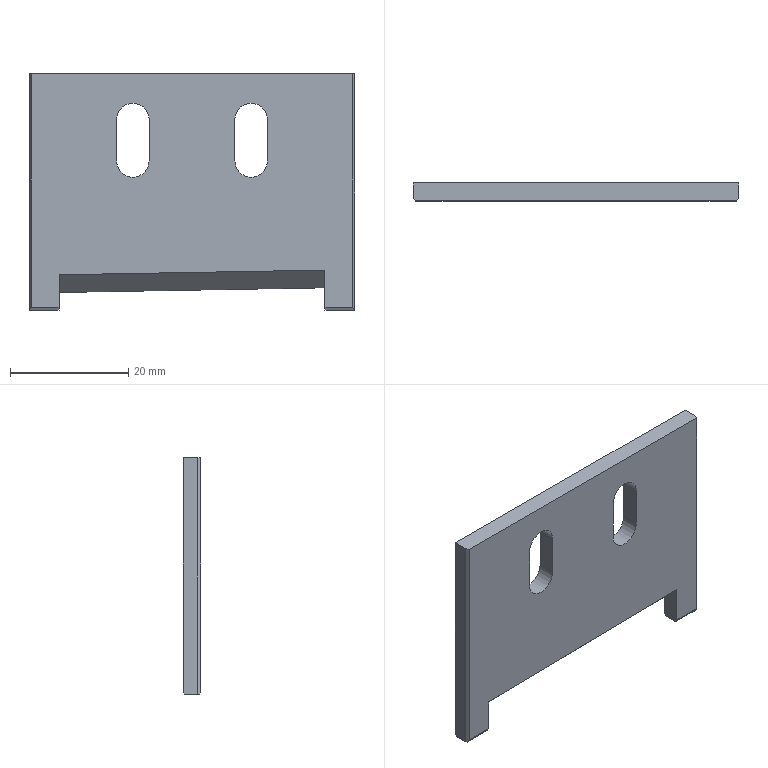Part | SolidWorks | features Chamfer 4, Draft 1, Extrusion 1, ICE 1 | 1 solid | 26 faces | box 55 x 3 x 40 mm | volume 5559 mm3 | plane 20 | cylinder 6 | commonest cylinder face diameters 5.5 x6
STEP:
#1=CARTESIAN_POINT('',(17.5,0.,-5.));
#2=VERTEX_POINT('',#1);
#3=CARTESIAN_POINT('',(20.25,0.,-7.75));
#4=VERTEX_POINT('',#3);
#5=CARTESIAN_POINT('',(17.5,0.,-7.75));
#6=DIRECTION('',(0.,1.,0.));
#7=DIRECTION('',(0.,0.,1.));
#8=AXIS2_PLACEMENT_3D('',#5,#6,#7);
#9=CIRCLE('',#8,2.75);
#10=EDGE_CURVE('',#2,#4,#9,.T.);
#11=ORIENTED_EDGE('',*,*,#10,.F.);
#12=CARTESIAN_POINT('',(17.5,3.,-5.));
#13=VERTEX_POINT('',#12);
#14=CARTESIAN_POINT('',(17.5,0.,-5.));
#15=DIRECTION('',(0.,1.,0.));
#16=VECTOR('',#15,1000.);
#17=LINE('',#14,#16);
#18=EDGE_CURVE('',#2,#13,#17,.T.);
#19=ORIENTED_EDGE('',*,*,#18,.T.);
#20=CARTESIAN_POINT('',(20.25,3.,-7.75));
#21=VERTEX_POINT('',#20);
#22=CARTESIAN_POINT('',(17.5,3.,-7.75));
#23=DIRECTION('',(0.,1.,0.));
#24=DIRECTION('',(0.,0.,1.));
#25=AXIS2_PLACEMENT_3D('',#22,#23,#24);
#26=CIRCLE('',#25,2.75);
#27=EDGE_CURVE('',#13,#21,#26,.T.);
#28=ORIENTED_EDGE('',*,*,#27,.T.);
#29=CARTESIAN_POINT('',(20.25,0.,-7.75));
#30=DIRECTION('',(0.,1.,0.));
#31=VECTOR('',#30,1000.);
#32=LINE('',#29,#31);
#33=EDGE_CURVE('',#4,#21,#32,.T.);
#34=ORIENTED_EDGE('',*,*,#33,.F.);
#35=EDGE_LOOP('',(#11,#19,#28,#34));
#36=FACE_OUTER_BOUND('',#35,.T.);
#37=CARTESIAN_POINT('',(17.5,0.,-7.75));
#38=DIRECTION('',(0.,1.,0.));
#39=DIRECTION('',(0.,0.,1.));
#40=AXIS2_PLACEMENT_3D('',#37,#38,#39);
#41=CYLINDRICAL_SURFACE('',#40,2.75);
#42=ADVANCED_FACE('',(#36),#41,.F.);
#43=CARTESIAN_POINT('',(37.5,0.,-5.));
#44=VERTEX_POINT('',#43);
#45=CARTESIAN_POINT('',(40.25,0.,-7.75));
#46=VERTEX_POINT('',#45);
#47=CARTESIAN_POINT('',(37.5,0.,-7.75));
#48=DIRECTION('',(0.,1.,0.));
#49=DIRECTION('',(0.,0.,1.));
#50=AXIS2_PLACEMENT_3D('',#47,#48,#49);
#51=CIRCLE('',#50,2.75);
#52=EDGE_CURVE('',#44,#46,#51,.T.);
#53=ORIENTED_EDGE('',*,*,#52,.F.);
#54=CARTESIAN_POINT('',(37.5,3.,-5.));
#55=VERTEX_POINT('',#54);
#56=CARTESIAN_POINT('',(37.5,0.,-5.));
#57=DIRECTION('',(0.,1.,0.));
#58=VECTOR('',#57,1000.);
#59=LINE('',#56,#58);
#60=EDGE_CURVE('',#44,#55,#59,.T.);
#61=ORIENTED_EDGE('',*,*,#60,.T.);
#62=CARTESIAN_POINT('',(40.25,3.,-7.75));
#63=VERTEX_POINT('',#62);
#64=CARTESIAN_POINT('',(37.5,3.,-7.75));
#65=DIRECTION('',(0.,1.,0.));
#66=DIRECTION('',(0.,0.,1.));
#67=AXIS2_PLACEMENT_3D('',#64,#65,#66);
#68=CIRCLE('',#67,2.75);
#69=EDGE_CURVE('',#55,#63,#68,.T.);
#70=ORIENTED_EDGE('',*,*,#69,.T.);
#71=CARTESIAN_POINT('',(40.25,0.,-7.75));
#72=DIRECTION('',(0.,1.,0.));
#73=VECTOR('',#72,1000.);
#74=LINE('',#71,#73);
#75=EDGE_CURVE('',#46,#63,#74,.T.);
#76=ORIENTED_EDGE('',*,*,#75,.F.);
#77=EDGE_LOOP('',(#53,#61,#70,#76));
#78=FACE_OUTER_BOUND('',#77,.T.);
#79=CARTESIAN_POINT('',(37.5,0.,-7.75));
#80=DIRECTION('',(0.,1.,0.));
#81=DIRECTION('',(0.,0.,1.));
#82=AXIS2_PLACEMENT_3D('',#79,#80,#81);
#83=CYLINDRICAL_SURFACE('',#82,2.75);
#84=ADVANCED_FACE('',(#78),#83,.F.);
#85=CARTESIAN_POINT('',(0.2887,0.,0.));
#86=VERTEX_POINT('',#85);
#87=CARTESIAN_POINT('',(54.711,0.,0.));
#88=VERTEX_POINT('',#87);
#89=CARTESIAN_POINT('',(0.,0.,0.));
#90=DIRECTION('',(1.,0.,0.));
#91=VECTOR('',#90,1000.);
#92=LINE('',#89,#91);
#93=EDGE_CURVE('',#86,#88,#92,.T.);
#94=ORIENTED_EDGE('',*,*,#93,.T.);
#95=CARTESIAN_POINT('',(55.,0.5,0.));
#96=VERTEX_POINT('',#95);
#97=CARTESIAN_POINT('',(55.,0.5,0.));
#98=DIRECTION('',(0.5,0.866,0.));
#99=VECTOR('',#98,1000.);
#100=LINE('',#97,#99);
#101=EDGE_CURVE('',#88,#96,#100,.T.);
#102=ORIENTED_EDGE('',*,*,#101,.T.);
#103=CARTESIAN_POINT('',(55.,3.,0.));
#104=VERTEX_POINT('',#103);
#105=CARTESIAN_POINT('',(55.,3.,0.));
#106=DIRECTION('',(0.,-1.,0.));
#107=VECTOR('',#106,1000.);
#108=LINE('',#105,#107);
#109=EDGE_CURVE('',#104,#96,#108,.T.);
#110=ORIENTED_EDGE('',*,*,#109,.F.);
#111=CARTESIAN_POINT('',(0.,3.,0.));
#112=VERTEX_POINT('',#111);
#113=CARTESIAN_POINT('',(0.,3.,0.));
#114=DIRECTION('',(1.,0.,0.));
#115=VECTOR('',#114,1000.);
#116=LINE('',#113,#115);
#117=EDGE_CURVE('',#112,#104,#116,.T.);
#118=ORIENTED_EDGE('',*,*,#117,.F.);
#119=CARTESIAN_POINT('',(0.,0.5,0.));
#120=VERTEX_POINT('',#119);
#121=CARTESIAN_POINT('',(0.,3.,0.));
#122=DIRECTION('',(0.,-1.,0.));
#123=VECTOR('',#122,1000.);
#124=LINE('',#121,#123);
#125=EDGE_CURVE('',#112,#120,#124,.T.);
#126=ORIENTED_EDGE('',*,*,#125,.T.);
#127=CARTESIAN_POINT('',(0.,0.5,0.));
#128=DIRECTION('',(0.5,-0.866,0.));
#129=VECTOR('',#128,1000.);
#130=LINE('',#127,#129);
#131=EDGE_CURVE('',#120,#86,#130,.T.);
#132=ORIENTED_EDGE('',*,*,#131,.T.);
#133=EDGE_LOOP('',(#94,#102,#110,#118,#126,#132));
#134=FACE_OUTER_BOUND('',#133,.T.);
#135=CARTESIAN_POINT('',(0.,3.,0.));
#136=DIRECTION('',(0.,0.,-1.));
#137=DIRECTION('',(-1.,0.,0.));
#138=AXIS2_PLACEMENT_3D('',#135,#136,#137);
#139=PLANE('',#138);
#140=ADVANCED_FACE('',(#134),#139,.F.);
#141=ORIENTED_EDGE('',*,*,#109,.T.);
#142=CARTESIAN_POINT('',(55.,0.5,-40.));
#143=VERTEX_POINT('',#142);
#144=CARTESIAN_POINT('',(55.,0.5,-39.5));
#145=DIRECTION('',(0.,0.,-1.));
#146=VECTOR('',#145,1000.);
#147=LINE('',#144,#146);
#148=EDGE_CURVE('',#96,#143,#147,.T.);
#149=ORIENTED_EDGE('',*,*,#148,.T.);
#150=CARTESIAN_POINT('',(55.,2.711,-40.));
#151=VERTEX_POINT('',#150);
#152=CARTESIAN_POINT('',(55.,3.,-40.));
#153=DIRECTION('',(0.,-1.,0.));
#154=VECTOR('',#153,1000.);
#155=LINE('',#152,#154);
#156=EDGE_CURVE('',#151,#143,#155,.T.);
#157=ORIENTED_EDGE('',*,*,#156,.F.);
#158=CARTESIAN_POINT('',(55.,3.,-39.5));
#159=VERTEX_POINT('',#158);
#160=CARTESIAN_POINT('',(55.,3.,-39.5));
#161=DIRECTION('',(0.,0.5,0.866));
#162=VECTOR('',#161,1000.);
#163=LINE('',#160,#162);
#164=EDGE_CURVE('',#151,#159,#163,.T.);
#165=ORIENTED_EDGE('',*,*,#164,.T.);
#166=CARTESIAN_POINT('',(55.,3.,0.));
#167=DIRECTION('',(0.,0.,-1.));
#168=VECTOR('',#167,1000.);
#169=LINE('',#166,#168);
#170=EDGE_CURVE('',#104,#159,#169,.T.);
#171=ORIENTED_EDGE('',*,*,#170,.F.);
#172=EDGE_LOOP('',(#141,#149,#157,#165,#171));
#173=FACE_OUTER_BOUND('',#172,.T.);
#174=CARTESIAN_POINT('',(55.,3.,-37.));
#175=DIRECTION('',(-1.,0.,0.));
#176=DIRECTION('',(0.,0.,1.));
#177=AXIS2_PLACEMENT_3D('',#174,#175,#176);
#178=PLANE('',#177);
#179=ADVANCED_FACE('',(#173),#178,.F.);
#180=ORIENTED_EDGE('',*,*,#156,.T.);
#181=CARTESIAN_POINT('',(54.878,0.2887,-40.));
#182=VERTEX_POINT('',#181);
#183=CARTESIAN_POINT('',(55.,0.5,-40.));
#184=DIRECTION('',(-0.5,-0.866,0.));
#185=VECTOR('',#184,1000.);
#186=LINE('',#183,#185);
#187=EDGE_CURVE('',#143,#182,#186,.T.);
#188=ORIENTED_EDGE('',*,*,#187,.T.);
#189=CARTESIAN_POINT('',(50.,0.2887,-40.));
#190=VERTEX_POINT('',#189);
#191=CARTESIAN_POINT('',(50.,0.2887,-40.));
#192=DIRECTION('',(-1.,0.,0.));
#193=VECTOR('',#192,1000.);
#194=LINE('',#191,#193);
#195=EDGE_CURVE('',#182,#190,#194,.T.);
#196=ORIENTED_EDGE('',*,*,#195,.T.);
#197=CARTESIAN_POINT('',(50.,2.711,-40.));
#198=VERTEX_POINT('',#197);
#199=CARTESIAN_POINT('',(50.,3.,-40.));
#200=DIRECTION('',(0.,-1.,0.));
#201=VECTOR('',#200,1000.);
#202=LINE('',#199,#201);
#203=EDGE_CURVE('',#198,#190,#202,.T.);
#204=ORIENTED_EDGE('',*,*,#203,.F.);
#205=CARTESIAN_POINT('',(55.,2.711,-40.));
#206=DIRECTION('',(1.,0.,0.));
#207=VECTOR('',#206,1000.);
#208=LINE('',#205,#207);
#209=EDGE_CURVE('',#198,#151,#208,.T.);
#210=ORIENTED_EDGE('',*,*,#209,.T.);
#211=EDGE_LOOP('',(#180,#188,#196,#204,#210));
#212=FACE_OUTER_BOUND('',#211,.T.);
#213=CARTESIAN_POINT('',(55.,3.,-40.));
#214=DIRECTION('',(0.,0.,1.));
#215=DIRECTION('',(1.,0.,0.));
#216=AXIS2_PLACEMENT_3D('',#213,#214,#215);
#217=PLANE('',#216);
#218=ADVANCED_FACE('',(#212),#217,.F.);
#219=CARTESIAN_POINT('',(50.,3.,-39.5));
#220=VERTEX_POINT('',#219);
#221=CARTESIAN_POINT('',(50.,3.,-36.215));
#222=VERTEX_POINT('',#221);
#223=CARTESIAN_POINT('',(50.,3.,-37.));
#224=DIRECTION('',(0.,0.,1.));
#225=VECTOR('',#224,1000.);
#226=LINE('',#223,#225);
#227=EDGE_CURVE('',#220,#222,#226,.T.);
#228=ORIENTED_EDGE('',*,*,#227,.F.);
#229=CARTESIAN_POINT('',(50.,3.,-39.5));
#230=DIRECTION('',(0.,-0.5,-0.866));
#231=VECTOR('',#230,1000.);
#232=LINE('',#229,#231);
#233=EDGE_CURVE('',#220,#198,#232,.T.);
#234=ORIENTED_EDGE('',*,*,#233,.T.);
#235=ORIENTED_EDGE('',*,*,#203,.T.);
#236=CARTESIAN_POINT('',(50.,0.,-39.5));
#237=VERTEX_POINT('',#236);
#238=CARTESIAN_POINT('',(50.,0.2887,-40.));
#239=DIRECTION('',(0.,-0.5,0.866));
#240=VECTOR('',#239,1000.);
#241=LINE('',#238,#240);
#242=EDGE_CURVE('',#190,#237,#241,.T.);
#243=ORIENTED_EDGE('',*,*,#242,.T.);
#244=CARTESIAN_POINT('',(50.,0.,-33.214));
#245=VERTEX_POINT('',#244);
#246=CARTESIAN_POINT('',(50.,0.,-37.));
#247=DIRECTION('',(0.,0.,1.));
#248=VECTOR('',#247,1000.);
#249=LINE('',#246,#248);
#250=EDGE_CURVE('',#237,#245,#249,.T.);
#251=ORIENTED_EDGE('',*,*,#250,.T.);
#252=CARTESIAN_POINT('',(50.,3.393,-36.607));
#253=DIRECTION('',(0.,0.7071,-0.7072));
#254=VECTOR('',#253,1000.);
#255=LINE('',#252,#254);
#256=EDGE_CURVE('',#245,#222,#255,.T.);
#257=ORIENTED_EDGE('',*,*,#256,.T.);
#258=EDGE_LOOP('',(#228,#234,#235,#243,#251,#257));
#259=FACE_OUTER_BOUND('',#258,.T.);
#260=CARTESIAN_POINT('',(50.,3.,-37.));
#261=DIRECTION('',(1.,0.,0.));
#262=DIRECTION('',(0.,0.,-1.));
#263=AXIS2_PLACEMENT_3D('',#260,#261,#262);
#264=PLANE('',#263);
#265=ADVANCED_FACE('',(#259),#264,.F.);
#266=CARTESIAN_POINT('',(5.,2.711,-40.));
#267=VERTEX_POINT('',#266);
#268=CARTESIAN_POINT('',(5.,0.2887,-40.));
#269=VERTEX_POINT('',#268);
#270=CARTESIAN_POINT('',(5.,3.,-40.));
#271=DIRECTION('',(0.,-1.,0.));
#272=VECTOR('',#271,1000.);
#273=LINE('',#270,#272);
#274=EDGE_CURVE('',#267,#269,#273,.T.);
#275=ORIENTED_EDGE('',*,*,#274,.F.);
#276=CARTESIAN_POINT('',(5.,3.,-39.5));
#277=VERTEX_POINT('',#276);
#278=CARTESIAN_POINT('',(5.,3.,-39.5));
#279=DIRECTION('',(0.,0.5,0.866));
#280=VECTOR('',#279,1000.);
#281=LINE('',#278,#280);
#282=EDGE_CURVE('',#267,#277,#281,.T.);
#283=ORIENTED_EDGE('',*,*,#282,.T.);
#284=CARTESIAN_POINT('',(5.,3.,-37.));
#285=VERTEX_POINT('',#284);
#286=CARTESIAN_POINT('',(5.,3.,-37.));
#287=DIRECTION('',(0.,0.,-1.));
#288=VECTOR('',#287,1000.);
#289=LINE('',#286,#288);
#290=EDGE_CURVE('',#285,#277,#289,.T.);
#291=ORIENTED_EDGE('',*,*,#290,.F.);
#292=CARTESIAN_POINT('',(5.,0.,-34.));
#293=VERTEX_POINT('',#292);
#294=CARTESIAN_POINT('',(5.,3.,-37.));
#295=DIRECTION('',(0.,-0.7071,0.7072));
#296=VECTOR('',#295,1000.);
#297=LINE('',#294,#296);
#298=EDGE_CURVE('',#285,#293,#297,.T.);
#299=ORIENTED_EDGE('',*,*,#298,.T.);
#300=CARTESIAN_POINT('',(5.,0.,-39.5));
#301=VERTEX_POINT('',#300);
#302=CARTESIAN_POINT('',(5.,0.,-37.));
#303=DIRECTION('',(0.,0.,-1.));
#304=VECTOR('',#303,1000.);
#305=LINE('',#302,#304);
#306=EDGE_CURVE('',#293,#301,#305,.T.);
#307=ORIENTED_EDGE('',*,*,#306,.T.);
#308=CARTESIAN_POINT('',(5.,0.2887,-40.));
#309=DIRECTION('',(0.,0.5,-0.866));
#310=VECTOR('',#309,1000.);
#311=LINE('',#308,#310);
#312=EDGE_CURVE('',#301,#269,#311,.T.);
#313=ORIENTED_EDGE('',*,*,#312,.T.);
#314=EDGE_LOOP('',(#275,#283,#291,#299,#307,#313));
#315=FACE_OUTER_BOUND('',#314,.T.);
#316=CARTESIAN_POINT('',(5.,3.,-37.));
#317=DIRECTION('',(-1.,0.,0.));
#318=DIRECTION('',(0.,0.,1.));
#319=AXIS2_PLACEMENT_3D('',#316,#317,#318);
#320=PLANE('',#319);
#321=ADVANCED_FACE('',(#315),#320,.F.);
#322=CARTESIAN_POINT('',(0.122,0.2887,-40.));
#323=VERTEX_POINT('',#322);
#324=CARTESIAN_POINT('',(0.,0.2887,-40.));
#325=DIRECTION('',(-1.,0.,0.));
#326=VECTOR('',#325,1000.);
#327=LINE('',#324,#326);
#328=EDGE_CURVE('',#269,#323,#327,.T.);
#329=ORIENTED_EDGE('',*,*,#328,.T.);
#330=CARTESIAN_POINT('',(0.,0.5,-40.));
#331=VERTEX_POINT('',#330);
#332=CARTESIAN_POINT('',(0.,0.5,-40.));
#333=DIRECTION('',(-0.5,0.866,0.));
#334=VECTOR('',#333,1000.);
#335=LINE('',#332,#334);
#336=EDGE_CURVE('',#323,#331,#335,.T.);
#337=ORIENTED_EDGE('',*,*,#336,.T.);
#338=CARTESIAN_POINT('',(0.,2.711,-40.));
#339=VERTEX_POINT('',#338);
#340=CARTESIAN_POINT('',(0.,3.,-40.));
#341=DIRECTION('',(0.,-1.,0.));
#342=VECTOR('',#341,1000.);
#343=LINE('',#340,#342);
#344=EDGE_CURVE('',#339,#331,#343,.T.);
#345=ORIENTED_EDGE('',*,*,#344,.F.);
#346=CARTESIAN_POINT('',(0.,2.711,-40.));
#347=DIRECTION('',(1.,0.,0.));
#348=VECTOR('',#347,1000.);
#349=LINE('',#346,#348);
#350=EDGE_CURVE('',#339,#267,#349,.T.);
#351=ORIENTED_EDGE('',*,*,#350,.T.);
#352=ORIENTED_EDGE('',*,*,#274,.T.);
#353=EDGE_LOOP('',(#329,#337,#345,#351,#352));
#354=FACE_OUTER_BOUND('',#353,.T.);
#355=CARTESIAN_POINT('',(0.,3.,-40.));
#356=DIRECTION('',(0.,0.,1.));
#357=DIRECTION('',(1.,0.,0.));
#358=AXIS2_PLACEMENT_3D('',#355,#356,#357);
#359=PLANE('',#358);
#360=ADVANCED_FACE('',(#354),#359,.F.);
#361=ORIENTED_EDGE('',*,*,#344,.T.);
#362=CARTESIAN_POINT('',(0.,0.5,0.));
#363=DIRECTION('',(0.,0.,1.));
#364=VECTOR('',#363,1000.);
#365=LINE('',#362,#364);
#366=EDGE_CURVE('',#331,#120,#365,.T.);
#367=ORIENTED_EDGE('',*,*,#366,.T.);
#368=ORIENTED_EDGE('',*,*,#125,.F.);
#369=CARTESIAN_POINT('',(0.,3.,-39.5));
#370=VERTEX_POINT('',#369);
#371=CARTESIAN_POINT('',(0.,3.,0.));
#372=DIRECTION('',(0.,0.,1.));
#373=VECTOR('',#372,1000.);
#374=LINE('',#371,#373);
#375=EDGE_CURVE('',#370,#112,#374,.T.);
#376=ORIENTED_EDGE('',*,*,#375,.F.);
#377=CARTESIAN_POINT('',(0.,3.,-39.5));
#378=DIRECTION('',(0.,-0.5,-0.866));
#379=VECTOR('',#378,1000.);
#380=LINE('',#377,#379);
#381=EDGE_CURVE('',#370,#339,#380,.T.);
#382=ORIENTED_EDGE('',*,*,#381,.T.);
#383=EDGE_LOOP('',(#361,#367,#368,#376,#382));
#384=FACE_OUTER_BOUND('',#383,.T.);
#385=CARTESIAN_POINT('',(0.,3.,-37.));
#386=DIRECTION('',(1.,0.,0.));
#387=DIRECTION('',(0.,0.,-1.));
#388=AXIS2_PLACEMENT_3D('',#385,#386,#387);
#389=PLANE('',#388);
#390=ADVANCED_FACE('',(#384),#389,.F.);
#391=CARTESIAN_POINT('',(14.75,3.,-14.75));
#392=VERTEX_POINT('',#391);
#393=CARTESIAN_POINT('',(14.75,3.,-7.75));
#394=VERTEX_POINT('',#393);
#395=CARTESIAN_POINT('',(14.75,3.,-14.75));
#396=DIRECTION('',(0.,0.,1.));
#397=VECTOR('',#396,1000.);
#398=LINE('',#395,#397);
#399=EDGE_CURVE('',#392,#394,#398,.T.);
#400=ORIENTED_EDGE('',*,*,#399,.F.);
#401=CARTESIAN_POINT('',(20.25,3.,-14.75));
#402=VERTEX_POINT('',#401);
#403=CARTESIAN_POINT('',(17.5,3.,-14.75));
#404=DIRECTION('',(0.,1.,0.));
#405=DIRECTION('',(0.,0.,1.));
#406=AXIS2_PLACEMENT_3D('',#403,#404,#405);
#407=CIRCLE('',#406,2.75);
#408=EDGE_CURVE('',#402,#392,#407,.T.);
#409=ORIENTED_EDGE('',*,*,#408,.F.);
#410=CARTESIAN_POINT('',(20.25,3.,-14.75));
#411=DIRECTION('',(0.,0.,-1.));
#412=VECTOR('',#411,1000.);
#413=LINE('',#410,#412);
#414=EDGE_CURVE('',#21,#402,#413,.T.);
#415=ORIENTED_EDGE('',*,*,#414,.F.);
#416=ORIENTED_EDGE('',*,*,#27,.F.);
#417=CARTESIAN_POINT('',(17.5,3.,-7.75));
#418=DIRECTION('',(0.,1.,0.));
#419=DIRECTION('',(0.,0.,1.));
#420=AXIS2_PLACEMENT_3D('',#417,#418,#419);
#421=CIRCLE('',#420,2.75);
#422=EDGE_CURVE('',#394,#13,#421,.T.);
#423=ORIENTED_EDGE('',*,*,#422,.F.);
#424=EDGE_LOOP('',(#400,#409,#415,#416,#423));
#425=FACE_BOUND('',#424,.T.);
#426=CARTESIAN_POINT('',(34.75,3.,-14.75));
#427=VERTEX_POINT('',#426);
#428=CARTESIAN_POINT('',(34.75,3.,-7.75));
#429=VERTEX_POINT('',#428);
#430=CARTESIAN_POINT('',(34.75,3.,-14.75));
#431=DIRECTION('',(0.,0.,1.));
#432=VECTOR('',#431,1000.);
#433=LINE('',#430,#432);
#434=EDGE_CURVE('',#427,#429,#433,.T.);
#435=ORIENTED_EDGE('',*,*,#434,.F.);
#436=CARTESIAN_POINT('',(40.25,3.,-14.75));
#437=VERTEX_POINT('',#436);
#438=CARTESIAN_POINT('',(37.5,3.,-14.75));
#439=DIRECTION('',(0.,1.,0.));
#440=DIRECTION('',(0.,0.,1.));
#441=AXIS2_PLACEMENT_3D('',#438,#439,#440);
#442=CIRCLE('',#441,2.75);
#443=EDGE_CURVE('',#437,#427,#442,.T.);
#444=ORIENTED_EDGE('',*,*,#443,.F.);
#445=CARTESIAN_POINT('',(40.25,3.,-14.75));
#446=DIRECTION('',(0.,0.,-1.));
#447=VECTOR('',#446,1000.);
#448=LINE('',#445,#447);
#449=EDGE_CURVE('',#63,#437,#448,.T.);
#450=ORIENTED_EDGE('',*,*,#449,.F.);
#451=ORIENTED_EDGE('',*,*,#69,.F.);
#452=CARTESIAN_POINT('',(37.5,3.,-7.75));
#453=DIRECTION('',(0.,1.,0.));
#454=DIRECTION('',(0.,0.,1.));
#455=AXIS2_PLACEMENT_3D('',#452,#453,#454);
#456=CIRCLE('',#455,2.75);
#457=EDGE_CURVE('',#429,#55,#456,.T.);
#458=ORIENTED_EDGE('',*,*,#457,.F.);
#459=EDGE_LOOP('',(#435,#444,#450,#451,#458));
#460=FACE_BOUND('',#459,.T.);
#461=ORIENTED_EDGE('',*,*,#290,.T.);
#462=CARTESIAN_POINT('',(0.,3.,-39.5));
#463=DIRECTION('',(-1.,0.,0.));
#464=VECTOR('',#463,1000.);
#465=LINE('',#462,#464);
#466=EDGE_CURVE('',#277,#370,#465,.T.);
#467=ORIENTED_EDGE('',*,*,#466,.T.);
#468=ORIENTED_EDGE('',*,*,#375,.T.);
#469=ORIENTED_EDGE('',*,*,#117,.T.);
#470=ORIENTED_EDGE('',*,*,#170,.T.);
#471=CARTESIAN_POINT('',(0.,3.,-39.5));
#472=DIRECTION('',(-1.,0.,0.));
#473=VECTOR('',#472,1000.);
#474=LINE('',#471,#473);
#475=EDGE_CURVE('',#159,#220,#474,.T.);
#476=ORIENTED_EDGE('',*,*,#475,.T.);
#477=ORIENTED_EDGE('',*,*,#227,.T.);
#478=CARTESIAN_POINT('',(0.6472,3.,-37.076));
#479=DIRECTION('',(-0.9998,0.,-0.01745));
#480=VECTOR('',#479,1000.);
#481=LINE('',#478,#480);
#482=EDGE_CURVE('',#222,#285,#481,.T.);
#483=ORIENTED_EDGE('',*,*,#482,.T.);
#484=EDGE_LOOP('',(#461,#467,#468,#469,#470,#476,#477,#483));
#485=FACE_OUTER_BOUND('',#484,.T.);
#486=CARTESIAN_POINT('',(0.,3.,0.));
#487=DIRECTION('',(0.,-1.,0.));
#488=DIRECTION('',(0.,0.,-1.));
#489=AXIS2_PLACEMENT_3D('',#486,#487,#488);
#490=PLANE('',#489);
#491=ADVANCED_FACE('',(#425,#460,#485),#490,.F.);
#492=CARTESIAN_POINT('',(20.25,0.,-14.75));
#493=VERTEX_POINT('',#492);
#494=CARTESIAN_POINT('',(14.75,0.,-14.75));
#495=VERTEX_POINT('',#494);
#496=CARTESIAN_POINT('',(17.5,0.,-14.75));
#497=DIRECTION('',(0.,1.,0.));
#498=DIRECTION('',(0.,0.,1.));
#499=AXIS2_PLACEMENT_3D('',#496,#497,#498);
#500=CIRCLE('',#499,2.75);
#501=EDGE_CURVE('',#493,#495,#500,.T.);
#502=ORIENTED_EDGE('',*,*,#501,.T.);
#503=CARTESIAN_POINT('',(14.75,0.,-7.75));
#504=VERTEX_POINT('',#503);
#505=CARTESIAN_POINT('',(14.75,0.,-14.75));
#506=DIRECTION('',(0.,0.,1.));
#507=VECTOR('',#506,1000.);
#508=LINE('',#505,#507);
#509=EDGE_CURVE('',#495,#504,#508,.T.);
#510=ORIENTED_EDGE('',*,*,#509,.T.);
#511=CARTESIAN_POINT('',(17.5,0.,-7.75));
#512=DIRECTION('',(0.,1.,0.));
#513=DIRECTION('',(0.,0.,1.));
#514=AXIS2_PLACEMENT_3D('',#511,#512,#513);
#515=CIRCLE('',#514,2.75);
#516=EDGE_CURVE('',#504,#2,#515,.T.);
#517=ORIENTED_EDGE('',*,*,#516,.T.);
#518=ORIENTED_EDGE('',*,*,#10,.T.);
#519=CARTESIAN_POINT('',(20.25,0.,-14.75));
#520=DIRECTION('',(0.,0.,-1.));
#521=VECTOR('',#520,1000.);
#522=LINE('',#519,#521);
#523=EDGE_CURVE('',#4,#493,#522,.T.);
#524=ORIENTED_EDGE('',*,*,#523,.T.);
#525=EDGE_LOOP('',(#502,#510,#517,#518,#524));
#526=FACE_BOUND('',#525,.T.);
#527=CARTESIAN_POINT('',(40.25,0.,-14.75));
#528=VERTEX_POINT('',#527);
#529=CARTESIAN_POINT('',(34.75,0.,-14.75));
#530=VERTEX_POINT('',#529);
#531=CARTESIAN_POINT('',(37.5,0.,-14.75));
#532=DIRECTION('',(0.,1.,0.));
#533=DIRECTION('',(0.,0.,1.));
#534=AXIS2_PLACEMENT_3D('',#531,#532,#533);
#535=CIRCLE('',#534,2.75);
#536=EDGE_CURVE('',#528,#530,#535,.T.);
#537=ORIENTED_EDGE('',*,*,#536,.T.);
#538=CARTESIAN_POINT('',(34.75,0.,-7.75));
#539=VERTEX_POINT('',#538);
#540=CARTESIAN_POINT('',(34.75,0.,-14.75));
#541=DIRECTION('',(0.,0.,1.));
#542=VECTOR('',#541,1000.);
#543=LINE('',#540,#542);
#544=EDGE_CURVE('',#530,#539,#543,.T.);
#545=ORIENTED_EDGE('',*,*,#544,.T.);
#546=CARTESIAN_POINT('',(37.5,0.,-7.75));
#547=DIRECTION('',(0.,1.,0.));
#548=DIRECTION('',(0.,0.,1.));
#549=AXIS2_PLACEMENT_3D('',#546,#547,#548);
#550=CIRCLE('',#549,2.75);
#551=EDGE_CURVE('',#539,#44,#550,.T.);
#552=ORIENTED_EDGE('',*,*,#551,.T.);
#553=ORIENTED_EDGE('',*,*,#52,.T.);
#554=CARTESIAN_POINT('',(40.25,0.,-14.75));
#555=DIRECTION('',(0.,0.,-1.));
#556=VECTOR('',#555,1000.);
#557=LINE('',#554,#556);
#558=EDGE_CURVE('',#46,#528,#557,.T.);
#559=ORIENTED_EDGE('',*,*,#558,.T.);
#560=EDGE_LOOP('',(#537,#545,#552,#553,#559));
#561=FACE_BOUND('',#560,.T.);
#562=CARTESIAN_POINT('',(54.711,0.,-39.5));
#563=VERTEX_POINT('',#562);
#564=CARTESIAN_POINT('',(55.,0.,-39.5));
#565=DIRECTION('',(1.,0.,0.));
#566=VECTOR('',#565,1000.);
#567=LINE('',#564,#566);
#568=EDGE_CURVE('',#237,#563,#567,.T.);
#569=ORIENTED_EDGE('',*,*,#568,.T.);
#570=CARTESIAN_POINT('',(54.711,0.,0.));
#571=DIRECTION('',(0.,0.,1.));
#572=VECTOR('',#571,1000.);
#573=LINE('',#570,#572);
#574=EDGE_CURVE('',#563,#88,#573,.T.);
#575=ORIENTED_EDGE('',*,*,#574,.T.);
#576=ORIENTED_EDGE('',*,*,#93,.F.);
#577=CARTESIAN_POINT('',(0.2887,0.,-39.5));
#578=VERTEX_POINT('',#577);
#579=CARTESIAN_POINT('',(0.2887,0.,-39.5));
#580=DIRECTION('',(0.,0.,-1.));
#581=VECTOR('',#580,1000.);
#582=LINE('',#579,#581);
#583=EDGE_CURVE('',#86,#578,#582,.T.);
#584=ORIENTED_EDGE('',*,*,#583,.T.);
#585=CARTESIAN_POINT('',(5.,0.,-39.5));
#586=DIRECTION('',(1.,0.,0.));
#587=VECTOR('',#586,1000.);
#588=LINE('',#585,#587);
#589=EDGE_CURVE('',#578,#301,#588,.T.);
#590=ORIENTED_EDGE('',*,*,#589,.T.);
#591=ORIENTED_EDGE('',*,*,#306,.F.);
#592=CARTESIAN_POINT('',(49.948,0.,-33.215));
#593=DIRECTION('',(0.9998,0.,0.01745));
#594=VECTOR('',#593,1000.);
#595=LINE('',#592,#594);
#596=EDGE_CURVE('',#293,#245,#595,.T.);
#597=ORIENTED_EDGE('',*,*,#596,.T.);
#598=ORIENTED_EDGE('',*,*,#250,.F.);
#599=EDGE_LOOP('',(#569,#575,#576,#584,#590,#591,#597,#598));
#600=FACE_OUTER_BOUND('',#599,.T.);
#601=CARTESIAN_POINT('',(0.,0.,0.));
#602=DIRECTION('',(0.,-1.,0.));
#603=DIRECTION('',(0.,0.,-1.));
#604=AXIS2_PLACEMENT_3D('',#601,#602,#603);
#605=PLANE('',#604);
#606=ADVANCED_FACE('',(#526,#561,#600),#605,.T.);
#607=ORIENTED_EDGE('',*,*,#443,.T.);
#608=CARTESIAN_POINT('',(34.75,0.,-14.75));
#609=DIRECTION('',(0.,1.,0.));
#610=VECTOR('',#609,1000.);
#611=LINE('',#608,#610);
#612=EDGE_CURVE('',#530,#427,#611,.T.);
#613=ORIENTED_EDGE('',*,*,#612,.F.);
#614=ORIENTED_EDGE('',*,*,#536,.F.);
#615=CARTESIAN_POINT('',(40.25,0.,-14.75));
#616=DIRECTION('',(0.,1.,0.));
#617=VECTOR('',#616,1000.);
#618=LINE('',#615,#617);
#619=EDGE_CURVE('',#528,#437,#618,.T.);
#620=ORIENTED_EDGE('',*,*,#619,.T.);
#621=EDGE_LOOP('',(#607,#613,#614,#620));
#622=FACE_OUTER_BOUND('',#621,.T.);
#623=CARTESIAN_POINT('',(37.5,0.,-14.75));
#624=DIRECTION('',(0.,1.,0.));
#625=DIRECTION('',(0.,0.,1.));
#626=AXIS2_PLACEMENT_3D('',#623,#624,#625);
#627=CYLINDRICAL_SURFACE('',#626,2.75);
#628=ADVANCED_FACE('',(#622),#627,.F.);
#629=ORIENTED_EDGE('',*,*,#449,.T.);
#630=ORIENTED_EDGE('',*,*,#619,.F.);
#631=ORIENTED_EDGE('',*,*,#558,.F.);
#632=ORIENTED_EDGE('',*,*,#75,.T.);
#633=EDGE_LOOP('',(#629,#630,#631,#632));
#634=FACE_OUTER_BOUND('',#633,.T.);
#635=CARTESIAN_POINT('',(40.25,0.,-14.75));
#636=DIRECTION('',(1.,0.,0.));
#637=DIRECTION('',(0.,0.,-1.));
#638=AXIS2_PLACEMENT_3D('',#635,#636,#637);
#639=PLANE('',#638);
#640=ADVANCED_FACE('',(#634),#639,.F.);
#641=ORIENTED_EDGE('',*,*,#60,.F.);
#642=ORIENTED_EDGE('',*,*,#551,.F.);
#643=CARTESIAN_POINT('',(34.75,0.,-7.75));
#644=DIRECTION('',(0.,1.,0.));
#645=VECTOR('',#644,1000.);
#646=LINE('',#643,#645);
#647=EDGE_CURVE('',#539,#429,#646,.T.);
#648=ORIENTED_EDGE('',*,*,#647,.T.);
#649=ORIENTED_EDGE('',*,*,#457,.T.);
#650=EDGE_LOOP('',(#641,#642,#648,#649));
#651=FACE_OUTER_BOUND('',#650,.T.);
#652=CARTESIAN_POINT('',(37.5,0.,-7.75));
#653=DIRECTION('',(0.,1.,0.));
#654=DIRECTION('',(0.,0.,1.));
#655=AXIS2_PLACEMENT_3D('',#652,#653,#654);
#656=CYLINDRICAL_SURFACE('',#655,2.75);
#657=ADVANCED_FACE('',(#651),#656,.F.);
#658=ORIENTED_EDGE('',*,*,#434,.T.);
#659=ORIENTED_EDGE('',*,*,#647,.F.);
#660=ORIENTED_EDGE('',*,*,#544,.F.);
#661=ORIENTED_EDGE('',*,*,#612,.T.);
#662=EDGE_LOOP('',(#658,#659,#660,#661));
#663=FACE_OUTER_BOUND('',#662,.T.);
#664=CARTESIAN_POINT('',(34.75,0.,-14.75));
#665=DIRECTION('',(-1.,0.,0.));
#666=DIRECTION('',(0.,0.,1.));
#667=AXIS2_PLACEMENT_3D('',#664,#665,#666);
#668=PLANE('',#667);
#669=ADVANCED_FACE('',(#663),#668,.F.);
#670=ORIENTED_EDGE('',*,*,#408,.T.);
#671=CARTESIAN_POINT('',(14.75,0.,-14.75));
#672=DIRECTION('',(0.,1.,0.));
#673=VECTOR('',#672,1000.);
#674=LINE('',#671,#673);
#675=EDGE_CURVE('',#495,#392,#674,.T.);
#676=ORIENTED_EDGE('',*,*,#675,.F.);
#677=ORIENTED_EDGE('',*,*,#501,.F.);
#678=CARTESIAN_POINT('',(20.25,0.,-14.75));
#679=DIRECTION('',(0.,1.,0.));
#680=VECTOR('',#679,1000.);
#681=LINE('',#678,#680);
#682=EDGE_CURVE('',#493,#402,#681,.T.);
#683=ORIENTED_EDGE('',*,*,#682,.T.);
#684=EDGE_LOOP('',(#670,#676,#677,#683));
#685=FACE_OUTER_BOUND('',#684,.T.);
#686=CARTESIAN_POINT('',(17.5,0.,-14.75));
#687=DIRECTION('',(0.,1.,0.));
#688=DIRECTION('',(0.,0.,1.));
#689=AXIS2_PLACEMENT_3D('',#686,#687,#688);
#690=CYLINDRICAL_SURFACE('',#689,2.75);
#691=ADVANCED_FACE('',(#685),#690,.F.);
#692=ORIENTED_EDGE('',*,*,#414,.T.);
#693=ORIENTED_EDGE('',*,*,#682,.F.);
#694=ORIENTED_EDGE('',*,*,#523,.F.);
#695=ORIENTED_EDGE('',*,*,#33,.T.);
#696=EDGE_LOOP('',(#692,#693,#694,#695));
#697=FACE_OUTER_BOUND('',#696,.T.);
#698=CARTESIAN_POINT('',(20.25,0.,-14.75));
#699=DIRECTION('',(1.,0.,0.));
#700=DIRECTION('',(0.,0.,-1.));
#701=AXIS2_PLACEMENT_3D('',#698,#699,#700);
#702=PLANE('',#701);
#703=ADVANCED_FACE('',(#697),#702,.F.);
#704=ORIENTED_EDGE('',*,*,#18,.F.);
#705=ORIENTED_EDGE('',*,*,#516,.F.);
#706=CARTESIAN_POINT('',(14.75,0.,-7.75));
#707=DIRECTION('',(0.,1.,0.));
#708=VECTOR('',#707,1000.);
#709=LINE('',#706,#708);
#710=EDGE_CURVE('',#504,#394,#709,.T.);
#711=ORIENTED_EDGE('',*,*,#710,.T.);
#712=ORIENTED_EDGE('',*,*,#422,.T.);
#713=EDGE_LOOP('',(#704,#705,#711,#712));
#714=FACE_OUTER_BOUND('',#713,.T.);
#715=CARTESIAN_POINT('',(17.5,0.,-7.75));
#716=DIRECTION('',(0.,1.,0.));
#717=DIRECTION('',(0.,0.,1.));
#718=AXIS2_PLACEMENT_3D('',#715,#716,#717);
#719=CYLINDRICAL_SURFACE('',#718,2.75);
#720=ADVANCED_FACE('',(#714),#719,.F.);
#721=ORIENTED_EDGE('',*,*,#399,.T.);
#722=ORIENTED_EDGE('',*,*,#710,.F.);
#723=ORIENTED_EDGE('',*,*,#509,.F.);
#724=ORIENTED_EDGE('',*,*,#675,.T.);
#725=EDGE_LOOP('',(#721,#722,#723,#724));
#726=FACE_OUTER_BOUND('',#725,.T.);
#727=CARTESIAN_POINT('',(14.75,0.,-14.75));
#728=DIRECTION('',(-1.,0.,0.));
#729=DIRECTION('',(0.,0.,1.));
#730=AXIS2_PLACEMENT_3D('',#727,#728,#729);
#731=PLANE('',#730);
#732=ADVANCED_FACE('',(#726),#731,.F.);
#733=ORIENTED_EDGE('',*,*,#256,.F.);
#734=ORIENTED_EDGE('',*,*,#596,.F.);
#735=ORIENTED_EDGE('',*,*,#298,.F.);
#736=ORIENTED_EDGE('',*,*,#482,.F.);
#737=EDGE_LOOP('',(#733,#734,#735,#736));
#738=FACE_OUTER_BOUND('',#737,.T.);
#739=CARTESIAN_POINT('',(5.,3.,-37.));
#740=DIRECTION('',(-0.01234,0.7071,0.707));
#741=DIRECTION('',(-0.9998,0.,-0.01745));
#742=AXIS2_PLACEMENT_3D('',#739,#740,#741);
#743=PLANE('',#742);
#744=ADVANCED_FACE('',(#738),#743,.F.);
#745=ORIENTED_EDGE('',*,*,#589,.F.);
#746=CARTESIAN_POINT('',(0.1126,0.3049,-40.028));
#747=DIRECTION('',(-0.2774,0.4804,-0.8321));
#748=VECTOR('',#747,1000.);
#749=LINE('',#746,#748);
#750=EDGE_CURVE('',#578,#323,#749,.T.);
#751=ORIENTED_EDGE('',*,*,#750,.T.);
#752=ORIENTED_EDGE('',*,*,#328,.F.);
#753=ORIENTED_EDGE('',*,*,#312,.F.);
#754=EDGE_LOOP('',(#745,#751,#752,#753));
#755=FACE_OUTER_BOUND('',#754,.T.);
#756=CARTESIAN_POINT('',(0.,0.2887,-40.));
#757=DIRECTION('',(0.,-0.866,-0.5));
#758=DIRECTION('',(1.,0.,0.));
#759=AXIS2_PLACEMENT_3D('',#756,#757,#758);
#760=PLANE('',#759);
#761=ADVANCED_FACE('',(#755),#760,.T.);
#762=ORIENTED_EDGE('',*,*,#195,.F.);
#763=CARTESIAN_POINT('',(54.887,0.3049,-40.028));
#764=DIRECTION('',(-0.2774,-0.4804,0.8321));
#765=VECTOR('',#764,1000.);
#766=LINE('',#763,#765);
#767=EDGE_CURVE('',#182,#563,#766,.T.);
#768=ORIENTED_EDGE('',*,*,#767,.T.);
#769=ORIENTED_EDGE('',*,*,#568,.F.);
#770=ORIENTED_EDGE('',*,*,#242,.F.);
#771=EDGE_LOOP('',(#762,#768,#769,#770));
#772=FACE_OUTER_BOUND('',#771,.T.);
#773=CARTESIAN_POINT('',(55.,0.2887,-40.));
#774=DIRECTION('',(0.,-0.866,-0.5));
#775=DIRECTION('',(1.,0.,0.));
#776=AXIS2_PLACEMENT_3D('',#773,#774,#775);
#777=PLANE('',#776);
#778=ADVANCED_FACE('',(#772),#777,.T.);
#779=ORIENTED_EDGE('',*,*,#282,.F.);
#780=ORIENTED_EDGE('',*,*,#350,.F.);
#781=ORIENTED_EDGE('',*,*,#381,.F.);
#782=ORIENTED_EDGE('',*,*,#466,.F.);
#783=EDGE_LOOP('',(#779,#780,#781,#782));
#784=FACE_OUTER_BOUND('',#783,.T.);
#785=CARTESIAN_POINT('',(0.,3.,-39.5));
#786=DIRECTION('',(0.,-0.866,0.5));
#787=DIRECTION('',(-1.,0.,0.));
#788=AXIS2_PLACEMENT_3D('',#785,#786,#787);
#789=PLANE('',#788);
#790=ADVANCED_FACE('',(#784),#789,.F.);
#791=ORIENTED_EDGE('',*,*,#164,.F.);
#792=ORIENTED_EDGE('',*,*,#209,.F.);
#793=ORIENTED_EDGE('',*,*,#233,.F.);
#794=ORIENTED_EDGE('',*,*,#475,.F.);
#795=EDGE_LOOP('',(#791,#792,#793,#794));
#796=FACE_OUTER_BOUND('',#795,.T.);
#797=CARTESIAN_POINT('',(0.,3.,-39.5));
#798=DIRECTION('',(0.,-0.866,0.5));
#799=DIRECTION('',(-1.,0.,0.));
#800=AXIS2_PLACEMENT_3D('',#797,#798,#799);
#801=PLANE('',#800);
#802=ADVANCED_FACE('',(#796),#801,.F.);
#803=ORIENTED_EDGE('',*,*,#101,.F.);
#804=ORIENTED_EDGE('',*,*,#574,.F.);
#805=ORIENTED_EDGE('',*,*,#767,.F.);
#806=ORIENTED_EDGE('',*,*,#187,.F.);
#807=ORIENTED_EDGE('',*,*,#148,.F.);
#808=EDGE_LOOP('',(#803,#804,#805,#806,#807));
#809=FACE_OUTER_BOUND('',#808,.T.);
#810=CARTESIAN_POINT('',(55.,0.5,-37.));
#811=DIRECTION('',(0.866,-0.5,0.));
#812=DIRECTION('',(0.,0.,1.));
#813=AXIS2_PLACEMENT_3D('',#810,#811,#812);
#814=PLANE('',#813);
#815=ADVANCED_FACE('',(#809),#814,.T.);
#816=ORIENTED_EDGE('',*,*,#750,.F.);
#817=ORIENTED_EDGE('',*,*,#583,.F.);
#818=ORIENTED_EDGE('',*,*,#131,.F.);
#819=ORIENTED_EDGE('',*,*,#366,.F.);
#820=ORIENTED_EDGE('',*,*,#336,.F.);
#821=EDGE_LOOP('',(#816,#817,#818,#819,#820));
#822=FACE_OUTER_BOUND('',#821,.T.);
#823=CARTESIAN_POINT('',(0.,0.5,-37.));
#824=DIRECTION('',(-0.866,-0.5,0.));
#825=DIRECTION('',(0.,0.,-1.));
#826=AXIS2_PLACEMENT_3D('',#823,#824,#825);
#827=PLANE('',#826);
#828=ADVANCED_FACE('',(#822),#827,.T.);
#829=CLOSED_SHELL('',(#42,#84,#140,#179,#218,#265,#321,#360,#390,#491,#606,#628,#640,#657,#669,#691,#703,#720,#732,#744,#761,#778,#790,#802,#815,#828));
#830=MANIFOLD_SOLID_BREP('',#829);
#831=CARTESIAN_POINT('',(0.,0.,0.));
#832=DIRECTION('',(0.,0.,1.));
#833=DIRECTION('',(1.,0.,0.));
#834=AXIS2_PLACEMENT_3D('',#831,#832,#833);
#835=(LENGTH_UNIT()NAMED_UNIT(*)SI_UNIT(.MILLI.,.METRE.));
#836=UNCERTAINTY_MEASURE_WITH_UNIT(LENGTH_MEASURE(0.00001),#835,'','');
#837=(NAMED_UNIT(*)PLANE_ANGLE_UNIT()SI_UNIT($,.RADIAN.));
#838=(NAMED_UNIT(*)SI_UNIT($,.STERADIAN.)SOLID_ANGLE_UNIT());
#839=(GEOMETRIC_REPRESENTATION_CONTEXT(3)GLOBAL_UNCERTAINTY_ASSIGNED_CONTEXT((#836))GLOBAL_UNIT_ASSIGNED_CONTEXT((#835,#837,#838))REPRESENTATION_CONTEXT('',''));
#840=ADVANCED_BREP_SHAPE_REPRESENTATION('',(#830,#834),#839);